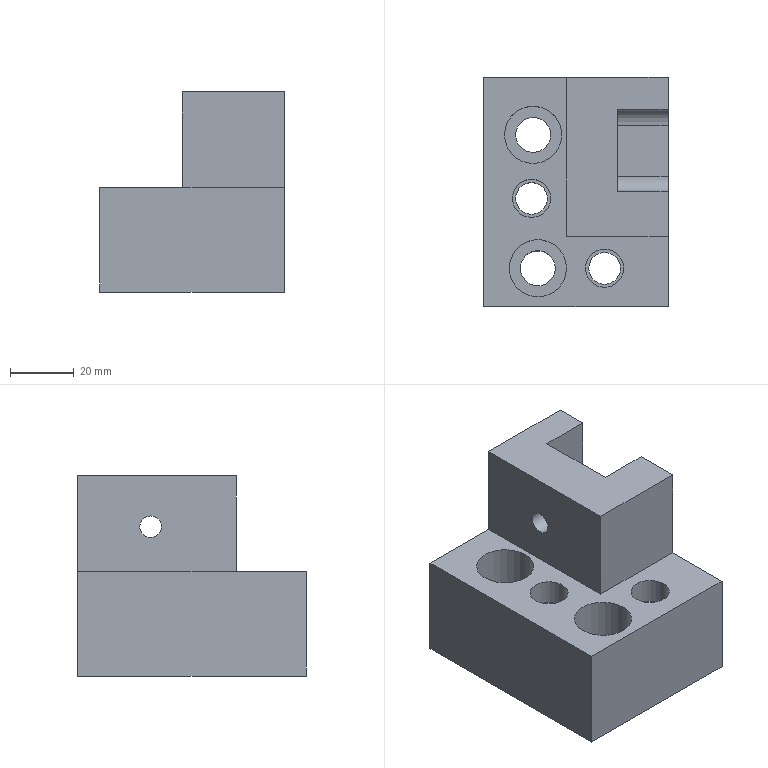Part | STEP file | gslz 2016.10.28-13_id458_x_t | 1 solid | 30 faces | box 58 x 72 x 63 mm | volume 149414 mm3 | plane 17 | cylinder 12 | cone 1 | commonest cylinder face diameters 10 x4 6.8 x2 11 x2 12 x2 18 x2